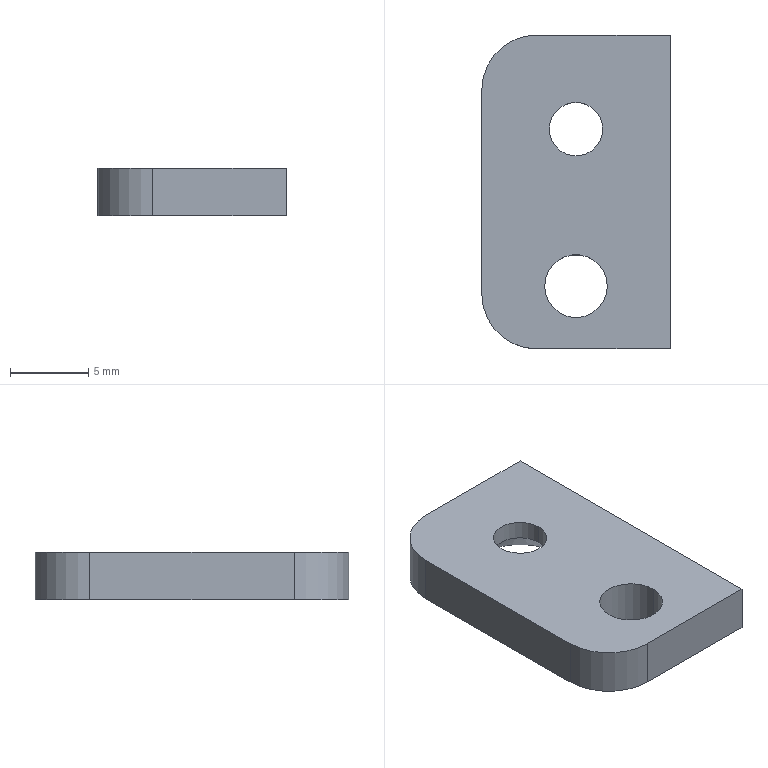Part | NX | features BREP 1 | 1 solid | 14 faces | box 12 x 20 x 3 mm | volume 615.879 mm3 | cylinder 6 | plane 6 | cone 2 | commonest cylinder face diameters 3.4 x2 4 x2 7 x2
STEP:
#1=CARTESIAN_POINT('',(-2.,-6.002,3.));
#2=VERTEX_POINT('',#1);
#3=CARTESIAN_POINT('',(-2.,-6.002,0.));
#4=VERTEX_POINT('',#3);
#5=CARTESIAN_POINT('',(-2.,-6.002,3.));
#6=DIRECTION('',(0.,0.,1.));
#7=VECTOR('',#6,1000.);
#8=LINE('',#5,#7);
#9=EDGE_CURVE('',#2,#4,#8,.F.);
#10=ORIENTED_EDGE('',*,*,#9,.T.);
#11=CARTESIAN_POINT('',(2.,-6.002,0.));
#12=VERTEX_POINT('',#11);
#13=CARTESIAN_POINT('',(0.,-6.002,0.));
#14=DIRECTION('',(0.,0.,1.));
#15=DIRECTION('',(1.,0.,0.));
#16=AXIS2_PLACEMENT_3D('',#13,#14,#15);
#17=CIRCLE('',#16,2.);
#18=EDGE_CURVE('',#12,#4,#17,.T.);
#19=ORIENTED_EDGE('',*,*,#18,.F.);
#20=CARTESIAN_POINT('',(2.,-6.002,3.));
#21=VERTEX_POINT('',#20);
#22=CARTESIAN_POINT('',(2.,-6.002,3.));
#23=DIRECTION('',(0.,0.,1.));
#24=VECTOR('',#23,1000.);
#25=LINE('',#22,#24);
#26=EDGE_CURVE('',#21,#12,#25,.F.);
#27=ORIENTED_EDGE('',*,*,#26,.F.);
#28=CARTESIAN_POINT('',(0.,-6.002,3.));
#29=DIRECTION('',(0.,0.,1.));
#30=DIRECTION('',(1.,0.,0.));
#31=AXIS2_PLACEMENT_3D('',#28,#29,#30);
#32=CIRCLE('',#31,2.);
#33=EDGE_CURVE('',#21,#2,#32,.T.);
#34=ORIENTED_EDGE('',*,*,#33,.T.);
#35=EDGE_LOOP('',(#10,#19,#27,#34));
#36=FACE_BOUND('',#35,.T.);
#37=CARTESIAN_POINT('',(0.,-6.002,3.));
#38=DIRECTION('',(0.,0.,1.));
#39=DIRECTION('',(1.,0.,0.));
#40=AXIS2_PLACEMENT_3D('',#37,#38,#39);
#41=CYLINDRICAL_SURFACE('',#40,2.);
#42=ADVANCED_FACE('',(#36),#41,.F.);
#43=CARTESIAN_POINT('',(1.7,4.,1.8));
#44=VERTEX_POINT('',#43);
#45=CARTESIAN_POINT('',(3.5,4.,0.));
#46=VERTEX_POINT('',#45);
#47=CARTESIAN_POINT('',(3.5,4.,0.));
#48=DIRECTION('',(0.7071,0.,-0.7071));
#49=VECTOR('',#48,1000.);
#50=LINE('',#47,#49);
#51=EDGE_CURVE('',#44,#46,#50,.T.);
#52=ORIENTED_EDGE('',*,*,#51,.F.);
#53=CARTESIAN_POINT('',(-1.7,4.,1.8));
#54=VERTEX_POINT('',#53);
#55=CARTESIAN_POINT('',(0.,4.,1.8));
#56=DIRECTION('',(0.,0.,-1.));
#57=DIRECTION('',(-1.,0.,0.));
#58=AXIS2_PLACEMENT_3D('',#55,#56,#57);
#59=CIRCLE('',#58,1.7);
#60=EDGE_CURVE('',#54,#44,#59,.T.);
#61=ORIENTED_EDGE('',*,*,#60,.F.);
#62=CARTESIAN_POINT('',(-3.5,4.,0.));
#63=VERTEX_POINT('',#62);
#64=CARTESIAN_POINT('',(-3.5,4.,0.));
#65=DIRECTION('',(-0.7071,0.,-0.7071));
#66=VECTOR('',#65,1000.);
#67=LINE('',#64,#66);
#68=EDGE_CURVE('',#54,#63,#67,.T.);
#69=ORIENTED_EDGE('',*,*,#68,.T.);
#70=CARTESIAN_POINT('',(0.,4.,0.));
#71=DIRECTION('',(0.,0.,-1.));
#72=DIRECTION('',(-1.,0.,0.));
#73=AXIS2_PLACEMENT_3D('',#70,#71,#72);
#74=CIRCLE('',#73,3.5);
#75=EDGE_CURVE('',#63,#46,#74,.T.);
#76=ORIENTED_EDGE('',*,*,#75,.T.);
#77=EDGE_LOOP('',(#52,#61,#69,#76));
#78=FACE_BOUND('',#77,.T.);
#79=CARTESIAN_POINT('',(0.,4.,0.));
#80=DIRECTION('',(0.,0.,-1.));
#81=DIRECTION('',(-1.,0.,0.));
#82=AXIS2_PLACEMENT_3D('',#79,#80,#81);
#83=CONICAL_SURFACE('',#82,3.5,0.7854);
#84=ADVANCED_FACE('',(#78),#83,.F.);
#85=CARTESIAN_POINT('',(1.7,4.,3.));
#86=VERTEX_POINT('',#85);
#87=CARTESIAN_POINT('',(1.7,4.,0.));
#88=DIRECTION('',(0.,0.,-1.));
#89=VECTOR('',#88,1000.);
#90=LINE('',#87,#89);
#91=EDGE_CURVE('',#86,#44,#90,.T.);
#92=ORIENTED_EDGE('',*,*,#91,.F.);
#93=CARTESIAN_POINT('',(-1.7,4.,3.));
#94=VERTEX_POINT('',#93);
#95=CARTESIAN_POINT('',(0.,4.,3.));
#96=DIRECTION('',(0.,0.,-1.));
#97=DIRECTION('',(-1.,0.,0.));
#98=AXIS2_PLACEMENT_3D('',#95,#96,#97);
#99=CIRCLE('',#98,1.7);
#100=EDGE_CURVE('',#94,#86,#99,.T.);
#101=ORIENTED_EDGE('',*,*,#100,.F.);
#102=CARTESIAN_POINT('',(-1.7,4.,0.));
#103=DIRECTION('',(0.,0.,-1.));
#104=VECTOR('',#103,1000.);
#105=LINE('',#102,#104);
#106=EDGE_CURVE('',#94,#54,#105,.T.);
#107=ORIENTED_EDGE('',*,*,#106,.T.);
#108=ORIENTED_EDGE('',*,*,#60,.T.);
#109=EDGE_LOOP('',(#92,#101,#107,#108));
#110=FACE_BOUND('',#109,.T.);
#111=CARTESIAN_POINT('',(0.,4.,0.));
#112=DIRECTION('',(0.,0.,-1.));
#113=DIRECTION('',(-1.,0.,0.));
#114=AXIS2_PLACEMENT_3D('',#111,#112,#113);
#115=CYLINDRICAL_SURFACE('',#114,1.7);
#116=ADVANCED_FACE('',(#110),#115,.F.);
#117=CARTESIAN_POINT('',(-2.5,10.,3.));
#118=VERTEX_POINT('',#117);
#119=CARTESIAN_POINT('',(-6.,6.5,3.));
#120=VERTEX_POINT('',#119);
#121=CARTESIAN_POINT('',(-2.5,6.5,3.));
#122=DIRECTION('',(0.,0.,1.));
#123=DIRECTION('',(-1.,0.,0.));
#124=AXIS2_PLACEMENT_3D('',#121,#122,#123);
#125=CIRCLE('',#124,3.5);
#126=EDGE_CURVE('',#118,#120,#125,.T.);
#127=ORIENTED_EDGE('',*,*,#126,.F.);
#128=CARTESIAN_POINT('',(-2.5,10.,0.));
#129=VERTEX_POINT('',#128);
#130=CARTESIAN_POINT('',(-2.5,10.,3.));
#131=DIRECTION('',(0.,0.,1.));
#132=VECTOR('',#131,1000.);
#133=LINE('',#130,#132);
#134=EDGE_CURVE('',#129,#118,#133,.T.);
#135=ORIENTED_EDGE('',*,*,#134,.F.);
#136=CARTESIAN_POINT('',(-6.,6.5,0.));
#137=VERTEX_POINT('',#136);
#138=CARTESIAN_POINT('',(-2.5,6.5,0.));
#139=DIRECTION('',(0.,0.,-1.));
#140=DIRECTION('',(-1.,0.,0.));
#141=AXIS2_PLACEMENT_3D('',#138,#139,#140);
#142=CIRCLE('',#141,3.5);
#143=EDGE_CURVE('',#137,#129,#142,.T.);
#144=ORIENTED_EDGE('',*,*,#143,.F.);
#145=CARTESIAN_POINT('',(-6.,6.5,3.));
#146=DIRECTION('',(0.,0.,-1.));
#147=VECTOR('',#146,1000.);
#148=LINE('',#145,#147);
#149=EDGE_CURVE('',#120,#137,#148,.T.);
#150=ORIENTED_EDGE('',*,*,#149,.F.);
#151=EDGE_LOOP('',(#127,#135,#144,#150));
#152=FACE_BOUND('',#151,.T.);
#153=CARTESIAN_POINT('',(-2.5,6.5,3.));
#154=DIRECTION('',(0.,0.,-1.));
#155=DIRECTION('',(-1.,0.,0.));
#156=AXIS2_PLACEMENT_3D('',#153,#154,#155);
#157=CYLINDRICAL_SURFACE('',#156,3.5);
#158=ADVANCED_FACE('',(#152),#157,.T.);
#159=CARTESIAN_POINT('',(-6.,-6.5,3.));
#160=VERTEX_POINT('',#159);
#161=CARTESIAN_POINT('',(-2.5,-10.,3.));
#162=VERTEX_POINT('',#161);
#163=CARTESIAN_POINT('',(-2.5,-6.5,3.));
#164=DIRECTION('',(0.,0.,1.));
#165=DIRECTION('',(-1.,0.,0.));
#166=AXIS2_PLACEMENT_3D('',#163,#164,#165);
#167=CIRCLE('',#166,3.5);
#168=EDGE_CURVE('',#160,#162,#167,.T.);
#169=ORIENTED_EDGE('',*,*,#168,.F.);
#170=CARTESIAN_POINT('',(-6.,-6.5,0.));
#171=VERTEX_POINT('',#170);
#172=CARTESIAN_POINT('',(-6.,-6.5,3.));
#173=DIRECTION('',(0.,0.,1.));
#174=VECTOR('',#173,1000.);
#175=LINE('',#172,#174);
#176=EDGE_CURVE('',#171,#160,#175,.T.);
#177=ORIENTED_EDGE('',*,*,#176,.F.);
#178=CARTESIAN_POINT('',(-2.5,-10.,0.));
#179=VERTEX_POINT('',#178);
#180=CARTESIAN_POINT('',(-2.5,-6.5,0.));
#181=DIRECTION('',(0.,0.,-1.));
#182=DIRECTION('',(-1.,0.,0.));
#183=AXIS2_PLACEMENT_3D('',#180,#181,#182);
#184=CIRCLE('',#183,3.5);
#185=EDGE_CURVE('',#179,#171,#184,.T.);
#186=ORIENTED_EDGE('',*,*,#185,.F.);
#187=CARTESIAN_POINT('',(-2.5,-10.,3.));
#188=DIRECTION('',(0.,0.,-1.));
#189=VECTOR('',#188,1000.);
#190=LINE('',#187,#189);
#191=EDGE_CURVE('',#162,#179,#190,.T.);
#192=ORIENTED_EDGE('',*,*,#191,.F.);
#193=EDGE_LOOP('',(#169,#177,#186,#192));
#194=FACE_BOUND('',#193,.T.);
#195=CARTESIAN_POINT('',(-2.5,-6.5,3.));
#196=DIRECTION('',(0.,0.,-1.));
#197=DIRECTION('',(-1.,0.,0.));
#198=AXIS2_PLACEMENT_3D('',#195,#196,#197);
#199=CYLINDRICAL_SURFACE('',#198,3.5);
#200=ADVANCED_FACE('',(#194),#199,.T.);
#201=CARTESIAN_POINT('',(6.,-10.,0.));
#202=VERTEX_POINT('',#201);
#203=CARTESIAN_POINT('',(-6.,-10.,0.));
#204=DIRECTION('',(1.,0.,0.));
#205=VECTOR('',#204,1000.);
#206=LINE('',#203,#205);
#207=EDGE_CURVE('',#179,#202,#206,.T.);
#208=ORIENTED_EDGE('',*,*,#207,.F.);
#209=ORIENTED_EDGE('',*,*,#185,.T.);
#210=CARTESIAN_POINT('',(-6.,-10.,0.));
#211=DIRECTION('',(0.,-1.,0.));
#212=VECTOR('',#211,1000.);
#213=LINE('',#210,#212);
#214=EDGE_CURVE('',#137,#171,#213,.T.);
#215=ORIENTED_EDGE('',*,*,#214,.F.);
#216=ORIENTED_EDGE('',*,*,#143,.T.);
#217=CARTESIAN_POINT('',(6.,10.,0.));
#218=VERTEX_POINT('',#217);
#219=CARTESIAN_POINT('',(-6.,10.,0.));
#220=DIRECTION('',(-1.,0.,0.));
#221=VECTOR('',#220,1000.);
#222=LINE('',#219,#221);
#223=EDGE_CURVE('',#218,#129,#222,.T.);
#224=ORIENTED_EDGE('',*,*,#223,.F.);
#225=CARTESIAN_POINT('',(6.,-10.,0.));
#226=DIRECTION('',(0.,1.,0.));
#227=VECTOR('',#226,1000.);
#228=LINE('',#225,#227);
#229=EDGE_CURVE('',#202,#218,#228,.T.);
#230=ORIENTED_EDGE('',*,*,#229,.F.);
#231=EDGE_LOOP('',(#208,#209,#215,#216,#224,#230));
#232=FACE_BOUND('',#231,.T.);
#233=ORIENTED_EDGE('',*,*,#75,.F.);
#234=CARTESIAN_POINT('',(0.,4.,0.));
#235=DIRECTION('',(0.,0.,-1.));
#236=DIRECTION('',(-1.,0.,0.));
#237=AXIS2_PLACEMENT_3D('',#234,#235,#236);
#238=CIRCLE('',#237,3.5);
#239=EDGE_CURVE('',#46,#63,#238,.T.);
#240=ORIENTED_EDGE('',*,*,#239,.F.);
#241=EDGE_LOOP('',(#233,#240));
#242=FACE_BOUND('',#241,.T.);
#243=ORIENTED_EDGE('',*,*,#18,.T.);
#244=CARTESIAN_POINT('',(0.,-6.002,0.));
#245=DIRECTION('',(0.,0.,1.));
#246=DIRECTION('',(1.,0.,0.));
#247=AXIS2_PLACEMENT_3D('',#244,#245,#246);
#248=CIRCLE('',#247,2.);
#249=EDGE_CURVE('',#4,#12,#248,.T.);
#250=ORIENTED_EDGE('',*,*,#249,.T.);
#251=EDGE_LOOP('',(#243,#250));
#252=FACE_BOUND('',#251,.T.);
#253=CARTESIAN_POINT('',(0.,0.,0.));
#254=DIRECTION('',(0.,0.,-1.));
#255=DIRECTION('',(-1.,0.,0.));
#256=AXIS2_PLACEMENT_3D('',#253,#254,#255);
#257=PLANE('',#256);
#258=ADVANCED_FACE('',(#232,#242,#252),#257,.T.);
#259=CARTESIAN_POINT('',(-6.,-10.,3.));
#260=DIRECTION('',(0.,-1.,0.));
#261=VECTOR('',#260,1000.);
#262=LINE('',#259,#261);
#263=EDGE_CURVE('',#120,#160,#262,.T.);
#264=ORIENTED_EDGE('',*,*,#263,.T.);
#265=ORIENTED_EDGE('',*,*,#168,.T.);
#266=CARTESIAN_POINT('',(6.,-10.,3.));
#267=VERTEX_POINT('',#266);
#268=CARTESIAN_POINT('',(-6.,-10.,3.));
#269=DIRECTION('',(1.,0.,0.));
#270=VECTOR('',#269,1000.);
#271=LINE('',#268,#270);
#272=EDGE_CURVE('',#162,#267,#271,.T.);
#273=ORIENTED_EDGE('',*,*,#272,.T.);
#274=CARTESIAN_POINT('',(6.,10.,3.));
#275=VERTEX_POINT('',#274);
#276=CARTESIAN_POINT('',(6.,-10.,3.));
#277=DIRECTION('',(0.,1.,0.));
#278=VECTOR('',#277,1000.);
#279=LINE('',#276,#278);
#280=EDGE_CURVE('',#267,#275,#279,.T.);
#281=ORIENTED_EDGE('',*,*,#280,.T.);
#282=CARTESIAN_POINT('',(-6.,10.,3.));
#283=DIRECTION('',(-1.,0.,0.));
#284=VECTOR('',#283,1000.);
#285=LINE('',#282,#284);
#286=EDGE_CURVE('',#275,#118,#285,.T.);
#287=ORIENTED_EDGE('',*,*,#286,.T.);
#288=ORIENTED_EDGE('',*,*,#126,.T.);
#289=EDGE_LOOP('',(#264,#265,#273,#281,#287,#288));
#290=FACE_BOUND('',#289,.T.);
#291=ORIENTED_EDGE('',*,*,#100,.T.);
#292=CARTESIAN_POINT('',(0.,4.,3.));
#293=DIRECTION('',(0.,0.,-1.));
#294=DIRECTION('',(-1.,0.,0.));
#295=AXIS2_PLACEMENT_3D('',#292,#293,#294);
#296=CIRCLE('',#295,1.7);
#297=EDGE_CURVE('',#86,#94,#296,.T.);
#298=ORIENTED_EDGE('',*,*,#297,.T.);
#299=EDGE_LOOP('',(#291,#298));
#300=FACE_BOUND('',#299,.T.);
#301=ORIENTED_EDGE('',*,*,#33,.F.);
#302=CARTESIAN_POINT('',(0.,-6.002,3.));
#303=DIRECTION('',(0.,0.,1.));
#304=DIRECTION('',(1.,0.,0.));
#305=AXIS2_PLACEMENT_3D('',#302,#303,#304);
#306=CIRCLE('',#305,2.);
#307=EDGE_CURVE('',#2,#21,#306,.T.);
#308=ORIENTED_EDGE('',*,*,#307,.F.);
#309=EDGE_LOOP('',(#301,#308));
#310=FACE_BOUND('',#309,.T.);
#311=CARTESIAN_POINT('',(0.,0.,3.));
#312=DIRECTION('',(0.,0.,-1.));
#313=DIRECTION('',(-1.,0.,0.));
#314=AXIS2_PLACEMENT_3D('',#311,#312,#313);
#315=PLANE('',#314);
#316=ADVANCED_FACE('',(#290,#300,#310),#315,.F.);
#317=ORIENTED_EDGE('',*,*,#272,.F.);
#318=ORIENTED_EDGE('',*,*,#191,.T.);
#319=ORIENTED_EDGE('',*,*,#207,.T.);
#320=CARTESIAN_POINT('',(6.,-10.,3.));
#321=DIRECTION('',(0.,0.,-1.));
#322=VECTOR('',#321,1000.);
#323=LINE('',#320,#322);
#324=EDGE_CURVE('',#267,#202,#323,.T.);
#325=ORIENTED_EDGE('',*,*,#324,.F.);
#326=EDGE_LOOP('',(#317,#318,#319,#325));
#327=FACE_BOUND('',#326,.T.);
#328=CARTESIAN_POINT('',(-6.,-10.,3.));
#329=DIRECTION('',(0.,1.,0.));
#330=DIRECTION('',(0.,0.,1.));
#331=AXIS2_PLACEMENT_3D('',#328,#329,#330);
#332=PLANE('',#331);
#333=ADVANCED_FACE('',(#327),#332,.F.);
#334=ORIENTED_EDGE('',*,*,#214,.T.);
#335=ORIENTED_EDGE('',*,*,#176,.T.);
#336=ORIENTED_EDGE('',*,*,#263,.F.);
#337=ORIENTED_EDGE('',*,*,#149,.T.);
#338=EDGE_LOOP('',(#334,#335,#336,#337));
#339=FACE_BOUND('',#338,.T.);
#340=CARTESIAN_POINT('',(-6.,-10.,3.));
#341=DIRECTION('',(1.,0.,0.));
#342=DIRECTION('',(0.,0.,-1.));
#343=AXIS2_PLACEMENT_3D('',#340,#341,#342);
#344=PLANE('',#343);
#345=ADVANCED_FACE('',(#339),#344,.F.);
#346=ORIENTED_EDGE('',*,*,#223,.T.);
#347=ORIENTED_EDGE('',*,*,#134,.T.);
#348=ORIENTED_EDGE('',*,*,#286,.F.);
#349=CARTESIAN_POINT('',(6.,10.,3.));
#350=DIRECTION('',(0.,0.,-1.));
#351=VECTOR('',#350,1000.);
#352=LINE('',#349,#351);
#353=EDGE_CURVE('',#275,#218,#352,.T.);
#354=ORIENTED_EDGE('',*,*,#353,.T.);
#355=EDGE_LOOP('',(#346,#347,#348,#354));
#356=FACE_BOUND('',#355,.T.);
#357=CARTESIAN_POINT('',(-6.,10.,3.));
#358=DIRECTION('',(0.,-1.,0.));
#359=DIRECTION('',(0.,0.,-1.));
#360=AXIS2_PLACEMENT_3D('',#357,#358,#359);
#361=PLANE('',#360);
#362=ADVANCED_FACE('',(#356),#361,.F.);
#363=ORIENTED_EDGE('',*,*,#229,.T.);
#364=ORIENTED_EDGE('',*,*,#353,.F.);
#365=ORIENTED_EDGE('',*,*,#280,.F.);
#366=ORIENTED_EDGE('',*,*,#324,.T.);
#367=EDGE_LOOP('',(#363,#364,#365,#366));
#368=FACE_BOUND('',#367,.T.);
#369=CARTESIAN_POINT('',(6.,-10.,3.));
#370=DIRECTION('',(-1.,0.,0.));
#371=DIRECTION('',(0.,0.,1.));
#372=AXIS2_PLACEMENT_3D('',#369,#370,#371);
#373=PLANE('',#372);
#374=ADVANCED_FACE('',(#368),#373,.F.);
#375=ORIENTED_EDGE('',*,*,#297,.F.);
#376=ORIENTED_EDGE('',*,*,#91,.T.);
#377=CARTESIAN_POINT('',(0.,4.,1.8));
#378=DIRECTION('',(0.,0.,-1.));
#379=DIRECTION('',(-1.,0.,0.));
#380=AXIS2_PLACEMENT_3D('',#377,#378,#379);
#381=CIRCLE('',#380,1.7);
#382=EDGE_CURVE('',#44,#54,#381,.T.);
#383=ORIENTED_EDGE('',*,*,#382,.T.);
#384=ORIENTED_EDGE('',*,*,#106,.F.);
#385=EDGE_LOOP('',(#375,#376,#383,#384));
#386=FACE_BOUND('',#385,.T.);
#387=CARTESIAN_POINT('',(0.,4.,0.));
#388=DIRECTION('',(0.,0.,-1.));
#389=DIRECTION('',(-1.,0.,0.));
#390=AXIS2_PLACEMENT_3D('',#387,#388,#389);
#391=CYLINDRICAL_SURFACE('',#390,1.7);
#392=ADVANCED_FACE('',(#386),#391,.F.);
#393=ORIENTED_EDGE('',*,*,#382,.F.);
#394=ORIENTED_EDGE('',*,*,#51,.T.);
#395=ORIENTED_EDGE('',*,*,#239,.T.);
#396=ORIENTED_EDGE('',*,*,#68,.F.);
#397=EDGE_LOOP('',(#393,#394,#395,#396));
#398=FACE_BOUND('',#397,.T.);
#399=CARTESIAN_POINT('',(0.,4.,0.));
#400=DIRECTION('',(0.,0.,-1.));
#401=DIRECTION('',(-1.,0.,0.));
#402=AXIS2_PLACEMENT_3D('',#399,#400,#401);
#403=CONICAL_SURFACE('',#402,3.5,0.7854);
#404=ADVANCED_FACE('',(#398),#403,.F.);
#405=ORIENTED_EDGE('',*,*,#249,.F.);
#406=ORIENTED_EDGE('',*,*,#9,.F.);
#407=ORIENTED_EDGE('',*,*,#307,.T.);
#408=ORIENTED_EDGE('',*,*,#26,.T.);
#409=EDGE_LOOP('',(#405,#406,#407,#408));
#410=FACE_BOUND('',#409,.T.);
#411=CARTESIAN_POINT('',(0.,-6.002,3.));
#412=DIRECTION('',(0.,0.,1.));
#413=DIRECTION('',(1.,0.,0.));
#414=AXIS2_PLACEMENT_3D('',#411,#412,#413);
#415=CYLINDRICAL_SURFACE('',#414,2.);
#416=ADVANCED_FACE('',(#410),#415,.F.);
#417=CLOSED_SHELL('',(#42,#84,#116,#158,#200,#258,#316,#333,#345,#362,#374,#392,#404,#416));
#418=MANIFOLD_SOLID_BREP('',#417);
#419=(LENGTH_UNIT()NAMED_UNIT(*)SI_UNIT(.MILLI.,.METRE.));
#420=UNCERTAINTY_MEASURE_WITH_UNIT(LENGTH_MEASURE(0.00001),#419,'','');
#421=(NAMED_UNIT(*)PLANE_ANGLE_UNIT()SI_UNIT($,.RADIAN.));
#422=(NAMED_UNIT(*)SI_UNIT($,.STERADIAN.)SOLID_ANGLE_UNIT());
#423=(GEOMETRIC_REPRESENTATION_CONTEXT(3)GLOBAL_UNCERTAINTY_ASSIGNED_CONTEXT((#420))GLOBAL_UNIT_ASSIGNED_CONTEXT((#419,#421,#422))REPRESENTATION_CONTEXT('',''));
#424=ADVANCED_BREP_SHAPE_REPRESENTATION('',(#418),#423);